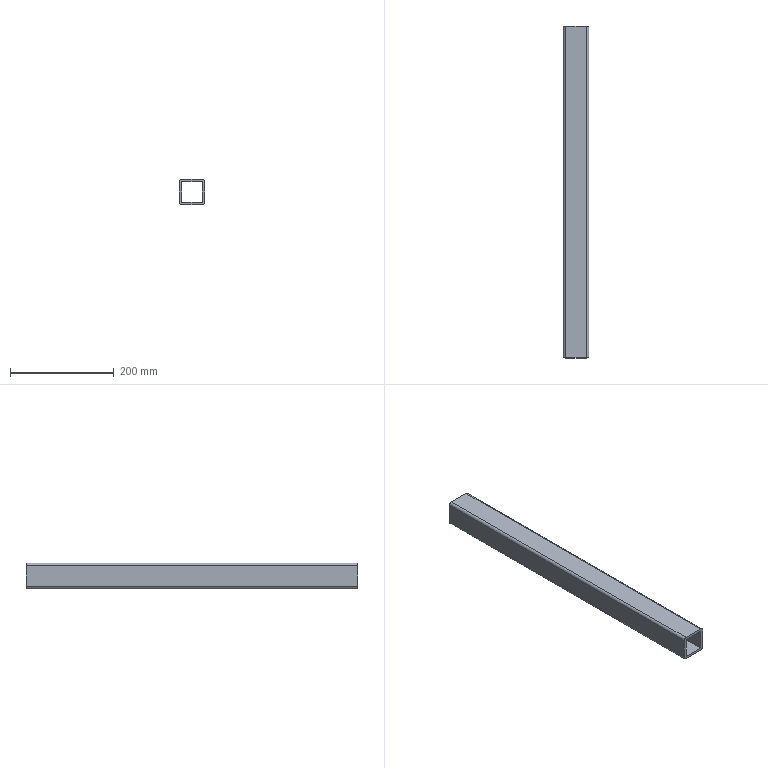Part | STEP file | 50x50x640 | 1 solid | 14 faces | box 50 x 640 x 50 mm | volume 562265 mm3 | plane 10 | cylinder 4 | commonest cylinder face diameters 10 x4
STEP:
#1=CARTESIAN_POINT('',(0.,0.,0.));
#2=DIRECTION('',(0.,0.,1.));
#3=DIRECTION('',(1.,0.,0.));
#4=AXIS2_PLACEMENT_3D('',#1,#2,#3);
#5=CARTESIAN_POINT('',(-758.5,-265.,-25.));
#6=VERTEX_POINT('',#5);
#7=CARTESIAN_POINT('',(-758.5,-265.,-65.));
#8=VERTEX_POINT('',#7);
#9=CARTESIAN_POINT('',(-758.5,-265.,-65.));
#10=DIRECTION('',(0.,0.,-1.));
#11=VECTOR('',#10,1.);
#12=LINE('',#9,#11);
#13=CARTESIAN_POINT('',(-758.5,845.,-65.));
#14=DIRECTION('',(-1.,0.,0.));
#15=DIRECTION('',(0.,0.,-1.));
#16=AXIS2_PLACEMENT_3D('',#13,#14,#15);
#17=PLANE('',#16);
#18=CARTESIAN_POINT('',(0.,1110.));
#19=DIRECTION('',(1.,0.));
#20=VECTOR('',#19,1.);
#21=LINE('',#18,#20);
#22=(GEOMETRIC_REPRESENTATION_CONTEXT(2)PARAMETRIC_REPRESENTATION_CONTEXT()REPRESENTATION_CONTEXT('',''));
#23=DEFINITIONAL_REPRESENTATION('',(#21),#22);
#24=PCURVE('',#17,#23);
#25=CARTESIAN_POINT('',(666.5,-265.,-65.));
#26=DIRECTION('',(0.,-1.,0.));
#27=DIRECTION('',(0.,0.,-1.));
#28=AXIS2_PLACEMENT_3D('',#25,#26,#27);
#29=PLANE('',#28);
#30=CARTESIAN_POINT('',(0.,-1425.));
#31=DIRECTION('',(1.,0.));
#32=VECTOR('',#31,1.);
#33=LINE('',#30,#32);
#34=(GEOMETRIC_REPRESENTATION_CONTEXT(2)PARAMETRIC_REPRESENTATION_CONTEXT()REPRESENTATION_CONTEXT('',''));
#35=DEFINITIONAL_REPRESENTATION('',(#33),#34);
#36=PCURVE('',#29,#35);
#37=SURFACE_CURVE('',#12,(#24,#36),.PCURVE_S1.);
#38=EDGE_CURVE('',#6,#8,#37,.T.);
#39=ORIENTED_EDGE('',*,*,#38,.F.);
#40=CARTESIAN_POINT('',(-758.5,375.,-25.));
#41=VERTEX_POINT('',#40);
#42=CARTESIAN_POINT('',(-758.5,845.,-25.));
#43=DIRECTION('',(0.,1.,0.));
#44=VECTOR('',#43,1.);
#45=LINE('',#42,#44);
#46=CARTESIAN_POINT('',(-40.,0.));
#47=DIRECTION('',(0.,-1.));
#48=VECTOR('',#47,1.);
#49=LINE('',#46,#48);
#50=(GEOMETRIC_REPRESENTATION_CONTEXT(2)PARAMETRIC_REPRESENTATION_CONTEXT()REPRESENTATION_CONTEXT('',''));
#51=DEFINITIONAL_REPRESENTATION('',(#49),#50);
#52=PCURVE('',#17,#51);
#53=CARTESIAN_POINT('',(-758.5,845.,-25.));
#54=DIRECTION('',(0.,0.,-1.));
#55=DIRECTION('',(1.,0.,0.));
#56=AXIS2_PLACEMENT_3D('',#53,#54,#55);
#57=PLANE('',#56);
#58=CARTESIAN_POINT('',(0.,0.));
#59=DIRECTION('',(0.,-1.));
#60=VECTOR('',#59,1.);
#61=LINE('',#58,#60);
#62=(GEOMETRIC_REPRESENTATION_CONTEXT(2)PARAMETRIC_REPRESENTATION_CONTEXT()REPRESENTATION_CONTEXT('',''));
#63=DEFINITIONAL_REPRESENTATION('',(#61),#62);
#64=PCURVE('',#57,#63);
#65=SURFACE_CURVE('',#45,(#52,#64),.PCURVE_S1.);
#66=EDGE_CURVE('',#6,#41,#65,.T.);
#67=ORIENTED_EDGE('',*,*,#66,.T.);
#68=CARTESIAN_POINT('',(-758.5,375.,-65.));
#69=VERTEX_POINT('',#68);
#70=CARTESIAN_POINT('',(-758.5,375.,-65.));
#71=DIRECTION('',(0.,0.,-1.));
#72=VECTOR('',#71,1.);
#73=LINE('',#70,#72);
#74=CARTESIAN_POINT('',(0.,470.));
#75=DIRECTION('',(1.,0.));
#76=VECTOR('',#75,1.);
#77=LINE('',#74,#76);
#78=(GEOMETRIC_REPRESENTATION_CONTEXT(2)PARAMETRIC_REPRESENTATION_CONTEXT()REPRESENTATION_CONTEXT('',''));
#79=DEFINITIONAL_REPRESENTATION('',(#77),#78);
#80=PCURVE('',#17,#79);
#81=CARTESIAN_POINT('',(-1003.5,375.,-65.));
#82=DIRECTION('',(0.,1.,0.));
#83=DIRECTION('',(0.,0.,-1.));
#84=AXIS2_PLACEMENT_3D('',#81,#82,#83);
#85=PLANE('',#84);
#86=CARTESIAN_POINT('',(0.,-245.));
#87=DIRECTION('',(1.,0.));
#88=VECTOR('',#87,1.);
#89=LINE('',#86,#88);
#90=(GEOMETRIC_REPRESENTATION_CONTEXT(2)PARAMETRIC_REPRESENTATION_CONTEXT()REPRESENTATION_CONTEXT('',''));
#91=DEFINITIONAL_REPRESENTATION('',(#89),#90);
#92=PCURVE('',#85,#91);
#93=SURFACE_CURVE('',#73,(#80,#92),.PCURVE_S1.);
#94=EDGE_CURVE('',#41,#69,#93,.T.);
#95=ORIENTED_EDGE('',*,*,#94,.T.);
#96=CARTESIAN_POINT('',(-758.5,845.,-65.));
#97=DIRECTION('',(0.,1.,0.));
#98=VECTOR('',#97,1.);
#99=LINE('',#96,#98);
#100=CARTESIAN_POINT('',(0.,0.));
#101=DIRECTION('',(0.,-1.));
#102=VECTOR('',#101,1.);
#103=LINE('',#100,#102);
#104=(GEOMETRIC_REPRESENTATION_CONTEXT(2)PARAMETRIC_REPRESENTATION_CONTEXT()REPRESENTATION_CONTEXT('',''));
#105=DEFINITIONAL_REPRESENTATION('',(#103),#104);
#106=PCURVE('',#17,#105);
#107=CARTESIAN_POINT('',(-798.5,845.,-65.));
#108=DIRECTION('',(0.,0.,1.));
#109=DIRECTION('',(-1.,0.,0.));
#110=AXIS2_PLACEMENT_3D('',#107,#108,#109);
#111=PLANE('',#110);
#112=CARTESIAN_POINT('',(-40.,0.));
#113=DIRECTION('',(0.,-1.));
#114=VECTOR('',#113,1.);
#115=LINE('',#112,#114);
#116=(GEOMETRIC_REPRESENTATION_CONTEXT(2)PARAMETRIC_REPRESENTATION_CONTEXT()REPRESENTATION_CONTEXT('',''));
#117=DEFINITIONAL_REPRESENTATION('',(#115),#116);
#118=PCURVE('',#111,#117);
#119=SURFACE_CURVE('',#99,(#106,#118),.PCURVE_S1.);
#120=EDGE_CURVE('',#8,#69,#119,.T.);
#121=ORIENTED_EDGE('',*,*,#120,.F.);
#122=EDGE_LOOP('',(#39,#67,#95,#121));
#123=FACE_BOUND('',#122,.T.);
#124=ADVANCED_FACE('',(#123),#17,.T.);
#125=CARTESIAN_POINT('',(-798.5,-265.,-25.));
#126=VERTEX_POINT('',#125);
#127=CARTESIAN_POINT('',(666.5,-265.,-25.));
#128=DIRECTION('',(1.,0.,0.));
#129=VECTOR('',#128,1.);
#130=LINE('',#127,#129);
#131=CARTESIAN_POINT('',(1425.,1110.));
#132=DIRECTION('',(1.,0.));
#133=VECTOR('',#132,1.);
#134=LINE('',#131,#133);
#135=(GEOMETRIC_REPRESENTATION_CONTEXT(2)PARAMETRIC_REPRESENTATION_CONTEXT()REPRESENTATION_CONTEXT('',''));
#136=DEFINITIONAL_REPRESENTATION('',(#134),#135);
#137=PCURVE('',#57,#136);
#138=CARTESIAN_POINT('',(-40.,0.));
#139=DIRECTION('',(0.,1.));
#140=VECTOR('',#139,1.);
#141=LINE('',#138,#140);
#142=(GEOMETRIC_REPRESENTATION_CONTEXT(2)PARAMETRIC_REPRESENTATION_CONTEXT()REPRESENTATION_CONTEXT('',''));
#143=DEFINITIONAL_REPRESENTATION('',(#141),#142);
#144=PCURVE('',#29,#143);
#145=SURFACE_CURVE('',#130,(#137,#144),.PCURVE_S1.);
#146=EDGE_CURVE('',#126,#6,#145,.T.);
#147=ORIENTED_EDGE('',*,*,#146,.F.);
#148=CARTESIAN_POINT('',(-798.5,375.,-25.));
#149=VERTEX_POINT('',#148);
#150=CARTESIAN_POINT('',(-798.5,845.,-25.));
#151=DIRECTION('',(0.,1.,0.));
#152=VECTOR('',#151,1.);
#153=LINE('',#150,#152);
#154=CARTESIAN_POINT('',(-40.,0.));
#155=DIRECTION('',(0.,-1.));
#156=VECTOR('',#155,1.);
#157=LINE('',#154,#156);
#158=(GEOMETRIC_REPRESENTATION_CONTEXT(2)PARAMETRIC_REPRESENTATION_CONTEXT()REPRESENTATION_CONTEXT('',''));
#159=DEFINITIONAL_REPRESENTATION('',(#157),#158);
#160=PCURVE('',#57,#159);
#161=CARTESIAN_POINT('',(-798.5,845.,-25.));
#162=DIRECTION('',(1.,0.,0.));
#163=DIRECTION('',(0.,0.,1.));
#164=AXIS2_PLACEMENT_3D('',#161,#162,#163);
#165=PLANE('',#164);
#166=CARTESIAN_POINT('',(0.,0.));
#167=DIRECTION('',(0.,-1.));
#168=VECTOR('',#167,1.);
#169=LINE('',#166,#168);
#170=(GEOMETRIC_REPRESENTATION_CONTEXT(2)PARAMETRIC_REPRESENTATION_CONTEXT()REPRESENTATION_CONTEXT('',''));
#171=DEFINITIONAL_REPRESENTATION('',(#169),#170);
#172=PCURVE('',#165,#171);
#173=SURFACE_CURVE('',#153,(#160,#172),.PCURVE_S1.);
#174=EDGE_CURVE('',#126,#149,#173,.T.);
#175=ORIENTED_EDGE('',*,*,#174,.T.);
#176=CARTESIAN_POINT('',(-1003.5,375.,-25.));
#177=DIRECTION('',(1.,0.,0.));
#178=VECTOR('',#177,1.);
#179=LINE('',#176,#178);
#180=CARTESIAN_POINT('',(-245.,470.));
#181=DIRECTION('',(1.,0.));
#182=VECTOR('',#181,1.);
#183=LINE('',#180,#182);
#184=(GEOMETRIC_REPRESENTATION_CONTEXT(2)PARAMETRIC_REPRESENTATION_CONTEXT()REPRESENTATION_CONTEXT('',''));
#185=DEFINITIONAL_REPRESENTATION('',(#183),#184);
#186=PCURVE('',#57,#185);
#187=CARTESIAN_POINT('',(-40.,0.));
#188=DIRECTION('',(0.,-1.));
#189=VECTOR('',#188,1.);
#190=LINE('',#187,#189);
#191=(GEOMETRIC_REPRESENTATION_CONTEXT(2)PARAMETRIC_REPRESENTATION_CONTEXT()REPRESENTATION_CONTEXT('',''));
#192=DEFINITIONAL_REPRESENTATION('',(#190),#191);
#193=PCURVE('',#85,#192);
#194=SURFACE_CURVE('',#179,(#186,#193),.PCURVE_S1.);
#195=EDGE_CURVE('',#149,#41,#194,.T.);
#196=ORIENTED_EDGE('',*,*,#195,.T.);
#197=ORIENTED_EDGE('',*,*,#66,.F.);
#198=EDGE_LOOP('',(#147,#175,#196,#197));
#199=FACE_BOUND('',#198,.T.);
#200=ADVANCED_FACE('',(#199),#57,.T.);
#201=CARTESIAN_POINT('',(-798.5,-265.,-65.));
#202=VERTEX_POINT('',#201);
#203=CARTESIAN_POINT('',(-798.5,-265.,-65.));
#204=DIRECTION('',(0.,0.,1.));
#205=VECTOR('',#204,1.);
#206=LINE('',#203,#205);
#207=CARTESIAN_POINT('',(-40.,1110.));
#208=DIRECTION('',(1.,0.));
#209=VECTOR('',#208,1.);
#210=LINE('',#207,#209);
#211=(GEOMETRIC_REPRESENTATION_CONTEXT(2)PARAMETRIC_REPRESENTATION_CONTEXT()REPRESENTATION_CONTEXT('',''));
#212=DEFINITIONAL_REPRESENTATION('',(#210),#211);
#213=PCURVE('',#165,#212);
#214=CARTESIAN_POINT('',(0.,-1465.));
#215=DIRECTION('',(-1.,0.));
#216=VECTOR('',#215,1.);
#217=LINE('',#214,#216);
#218=(GEOMETRIC_REPRESENTATION_CONTEXT(2)PARAMETRIC_REPRESENTATION_CONTEXT()REPRESENTATION_CONTEXT('',''));
#219=DEFINITIONAL_REPRESENTATION('',(#217),#218);
#220=PCURVE('',#29,#219);
#221=SURFACE_CURVE('',#206,(#213,#220),.PCURVE_S1.);
#222=EDGE_CURVE('',#202,#126,#221,.T.);
#223=ORIENTED_EDGE('',*,*,#222,.F.);
#224=CARTESIAN_POINT('',(-798.5,375.,-65.));
#225=VERTEX_POINT('',#224);
#226=CARTESIAN_POINT('',(-798.5,845.,-65.));
#227=DIRECTION('',(0.,1.,0.));
#228=VECTOR('',#227,1.);
#229=LINE('',#226,#228);
#230=CARTESIAN_POINT('',(-40.,0.));
#231=DIRECTION('',(0.,-1.));
#232=VECTOR('',#231,1.);
#233=LINE('',#230,#232);
#234=(GEOMETRIC_REPRESENTATION_CONTEXT(2)PARAMETRIC_REPRESENTATION_CONTEXT()REPRESENTATION_CONTEXT('',''));
#235=DEFINITIONAL_REPRESENTATION('',(#233),#234);
#236=PCURVE('',#165,#235);
#237=CARTESIAN_POINT('',(0.,0.));
#238=DIRECTION('',(0.,-1.));
#239=VECTOR('',#238,1.);
#240=LINE('',#237,#239);
#241=(GEOMETRIC_REPRESENTATION_CONTEXT(2)PARAMETRIC_REPRESENTATION_CONTEXT()REPRESENTATION_CONTEXT('',''));
#242=DEFINITIONAL_REPRESENTATION('',(#240),#241);
#243=PCURVE('',#111,#242);
#244=SURFACE_CURVE('',#229,(#236,#243),.PCURVE_S1.);
#245=EDGE_CURVE('',#202,#225,#244,.T.);
#246=ORIENTED_EDGE('',*,*,#245,.T.);
#247=CARTESIAN_POINT('',(-798.5,375.,-65.));
#248=DIRECTION('',(0.,0.,1.));
#249=VECTOR('',#248,1.);
#250=LINE('',#247,#249);
#251=CARTESIAN_POINT('',(-40.,470.));
#252=DIRECTION('',(1.,0.));
#253=VECTOR('',#252,1.);
#254=LINE('',#251,#253);
#255=(GEOMETRIC_REPRESENTATION_CONTEXT(2)PARAMETRIC_REPRESENTATION_CONTEXT()REPRESENTATION_CONTEXT('',''));
#256=DEFINITIONAL_REPRESENTATION('',(#254),#255);
#257=PCURVE('',#165,#256);
#258=CARTESIAN_POINT('',(0.,-205.));
#259=DIRECTION('',(-1.,0.));
#260=VECTOR('',#259,1.);
#261=LINE('',#258,#260);
#262=(GEOMETRIC_REPRESENTATION_CONTEXT(2)PARAMETRIC_REPRESENTATION_CONTEXT()REPRESENTATION_CONTEXT('',''));
#263=DEFINITIONAL_REPRESENTATION('',(#261),#262);
#264=PCURVE('',#85,#263);
#265=SURFACE_CURVE('',#250,(#257,#264),.PCURVE_S1.);
#266=EDGE_CURVE('',#225,#149,#265,.T.);
#267=ORIENTED_EDGE('',*,*,#266,.T.);
#268=ORIENTED_EDGE('',*,*,#174,.F.);
#269=EDGE_LOOP('',(#223,#246,#267,#268));
#270=FACE_BOUND('',#269,.T.);
#271=ADVANCED_FACE('',(#270),#165,.T.);
#272=CARTESIAN_POINT('',(-753.5,-265.,-65.));
#273=VERTEX_POINT('',#272);
#274=CARTESIAN_POINT('',(-753.5,-265.,-25.));
#275=VERTEX_POINT('',#274);
#276=CARTESIAN_POINT('',(-753.5,-265.,-65.));
#277=DIRECTION('',(0.,0.,1.));
#278=VECTOR('',#277,1.);
#279=LINE('',#276,#278);
#280=CARTESIAN_POINT('',(-753.5,845.,-25.));
#281=DIRECTION('',(1.,0.,0.));
#282=DIRECTION('',(0.,0.,1.));
#283=AXIS2_PLACEMENT_3D('',#280,#281,#282);
#284=PLANE('',#283);
#285=CARTESIAN_POINT('',(-40.,1110.));
#286=DIRECTION('',(1.,0.));
#287=VECTOR('',#286,1.);
#288=LINE('',#285,#287);
#289=(GEOMETRIC_REPRESENTATION_CONTEXT(2)PARAMETRIC_REPRESENTATION_CONTEXT()REPRESENTATION_CONTEXT('',''));
#290=DEFINITIONAL_REPRESENTATION('',(#288),#289);
#291=PCURVE('',#284,#290);
#292=CARTESIAN_POINT('',(0.,-1420.));
#293=DIRECTION('',(-1.,0.));
#294=VECTOR('',#293,1.);
#295=LINE('',#292,#294);
#296=(GEOMETRIC_REPRESENTATION_CONTEXT(2)PARAMETRIC_REPRESENTATION_CONTEXT()REPRESENTATION_CONTEXT('',''));
#297=DEFINITIONAL_REPRESENTATION('',(#295),#296);
#298=PCURVE('',#29,#297);
#299=SURFACE_CURVE('',#279,(#291,#298),.PCURVE_S1.);
#300=EDGE_CURVE('',#273,#275,#299,.T.);
#301=ORIENTED_EDGE('',*,*,#300,.F.);
#302=CARTESIAN_POINT('',(-753.5,375.,-65.));
#303=VERTEX_POINT('',#302);
#304=CARTESIAN_POINT('',(-753.5,845.,-65.));
#305=DIRECTION('',(0.,1.,0.));
#306=VECTOR('',#305,1.);
#307=LINE('',#304,#306);
#308=CARTESIAN_POINT('',(-40.,0.));
#309=DIRECTION('',(0.,-1.));
#310=VECTOR('',#309,1.);
#311=LINE('',#308,#310);
#312=(GEOMETRIC_REPRESENTATION_CONTEXT(2)PARAMETRIC_REPRESENTATION_CONTEXT()REPRESENTATION_CONTEXT('',''));
#313=DEFINITIONAL_REPRESENTATION('',(#311),#312);
#314=PCURVE('',#284,#313);
#315=CARTESIAN_POINT('',(-758.5,845.,-65.));
#316=DIRECTION('',(0.,-1.,0.));
#317=DIRECTION('',(0.,0.,-1.));
#318=AXIS2_PLACEMENT_3D('',#315,#316,#317);
#319=CYLINDRICAL_SURFACE('',#318,5.);
#320=CARTESIAN_POINT('',(1.571,0.));
#321=DIRECTION('',(0.,-1.));
#322=VECTOR('',#321,1.);
#323=LINE('',#320,#322);
#324=(GEOMETRIC_REPRESENTATION_CONTEXT(2)PARAMETRIC_REPRESENTATION_CONTEXT()REPRESENTATION_CONTEXT('',''));
#325=DEFINITIONAL_REPRESENTATION('',(#323),#324);
#326=PCURVE('',#319,#325);
#327=SURFACE_CURVE('',#307,(#314,#326),.PCURVE_S1.);
#328=EDGE_CURVE('',#273,#303,#327,.T.);
#329=ORIENTED_EDGE('',*,*,#328,.T.);
#330=CARTESIAN_POINT('',(-753.5,375.,-25.));
#331=VERTEX_POINT('',#330);
#332=CARTESIAN_POINT('',(-753.5,375.,-65.));
#333=DIRECTION('',(0.,0.,1.));
#334=VECTOR('',#333,1.);
#335=LINE('',#332,#334);
#336=CARTESIAN_POINT('',(-40.,470.));
#337=DIRECTION('',(1.,0.));
#338=VECTOR('',#337,1.);
#339=LINE('',#336,#338);
#340=(GEOMETRIC_REPRESENTATION_CONTEXT(2)PARAMETRIC_REPRESENTATION_CONTEXT()REPRESENTATION_CONTEXT('',''));
#341=DEFINITIONAL_REPRESENTATION('',(#339),#340);
#342=PCURVE('',#284,#341);
#343=CARTESIAN_POINT('',(0.,-250.));
#344=DIRECTION('',(-1.,0.));
#345=VECTOR('',#344,1.);
#346=LINE('',#343,#345);
#347=(GEOMETRIC_REPRESENTATION_CONTEXT(2)PARAMETRIC_REPRESENTATION_CONTEXT()REPRESENTATION_CONTEXT('',''));
#348=DEFINITIONAL_REPRESENTATION('',(#346),#347);
#349=PCURVE('',#85,#348);
#350=SURFACE_CURVE('',#335,(#342,#349),.PCURVE_S1.);
#351=EDGE_CURVE('',#303,#331,#350,.T.);
#352=ORIENTED_EDGE('',*,*,#351,.T.);
#353=CARTESIAN_POINT('',(-753.5,845.,-25.));
#354=DIRECTION('',(0.,1.,0.));
#355=VECTOR('',#354,1.);
#356=LINE('',#353,#355);
#357=CARTESIAN_POINT('',(0.,0.));
#358=DIRECTION('',(0.,-1.));
#359=VECTOR('',#358,1.);
#360=LINE('',#357,#359);
#361=(GEOMETRIC_REPRESENTATION_CONTEXT(2)PARAMETRIC_REPRESENTATION_CONTEXT()REPRESENTATION_CONTEXT('',''));
#362=DEFINITIONAL_REPRESENTATION('',(#360),#361);
#363=PCURVE('',#284,#362);
#364=CARTESIAN_POINT('',(-758.5,845.,-25.));
#365=DIRECTION('',(0.,-1.,0.));
#366=DIRECTION('',(0.,0.,-1.));
#367=AXIS2_PLACEMENT_3D('',#364,#365,#366);
#368=CYLINDRICAL_SURFACE('',#367,5.);
#369=CARTESIAN_POINT('',(1.571,0.));
#370=DIRECTION('',(0.,-1.));
#371=VECTOR('',#370,1.);
#372=LINE('',#369,#371);
#373=(GEOMETRIC_REPRESENTATION_CONTEXT(2)PARAMETRIC_REPRESENTATION_CONTEXT()REPRESENTATION_CONTEXT('',''));
#374=DEFINITIONAL_REPRESENTATION('',(#372),#373);
#375=PCURVE('',#368,#374);
#376=SURFACE_CURVE('',#356,(#363,#375),.PCURVE_S1.);
#377=EDGE_CURVE('',#275,#331,#376,.T.);
#378=ORIENTED_EDGE('',*,*,#377,.F.);
#379=EDGE_LOOP('',(#301,#329,#352,#378));
#380=FACE_BOUND('',#379,.T.);
#381=ADVANCED_FACE('',(#380),#284,.T.);
#382=CARTESIAN_POINT('',(-758.5,-265.,-70.));
#383=VERTEX_POINT('',#382);
#384=CARTESIAN_POINT('',(-758.5,-265.,-65.));
#385=DIRECTION('',(0.,-1.,0.));
#386=DIRECTION('',(0.,0.,-1.));
#387=AXIS2_PLACEMENT_3D('',#384,#385,#386);
#388=CIRCLE('',#387,5.);
#389=CARTESIAN_POINT('',(0.,1110.));
#390=DIRECTION('',(1.,0.));
#391=VECTOR('',#390,1.);
#392=LINE('',#389,#391);
#393=(GEOMETRIC_REPRESENTATION_CONTEXT(2)PARAMETRIC_REPRESENTATION_CONTEXT()REPRESENTATION_CONTEXT('',''));
#394=DEFINITIONAL_REPRESENTATION('',(#392),#393);
#395=PCURVE('',#319,#394);
#396=CARTESIAN_POINT('',(0.,-1425.));
#397=DIRECTION('',(1.,0.));
#398=AXIS2_PLACEMENT_2D('',#396,#397);
#399=CIRCLE('',#398,5.);
#400=(GEOMETRIC_REPRESENTATION_CONTEXT(2)PARAMETRIC_REPRESENTATION_CONTEXT()REPRESENTATION_CONTEXT('',''));
#401=DEFINITIONAL_REPRESENTATION('',(#399),#400);
#402=PCURVE('',#29,#401);
#403=SURFACE_CURVE('',#388,(#395,#402),.PCURVE_S1.);
#404=EDGE_CURVE('',#383,#273,#403,.T.);
#405=ORIENTED_EDGE('',*,*,#404,.F.);
#406=CARTESIAN_POINT('',(-758.5,375.,-70.));
#407=VERTEX_POINT('',#406);
#408=CARTESIAN_POINT('',(-758.5,845.,-70.));
#409=DIRECTION('',(0.,1.,0.));
#410=VECTOR('',#409,1.);
#411=LINE('',#408,#410);
#412=CARTESIAN_POINT('',(0.,0.));
#413=DIRECTION('',(0.,-1.));
#414=VECTOR('',#413,1.);
#415=LINE('',#412,#414);
#416=(GEOMETRIC_REPRESENTATION_CONTEXT(2)PARAMETRIC_REPRESENTATION_CONTEXT()REPRESENTATION_CONTEXT('',''));
#417=DEFINITIONAL_REPRESENTATION('',(#415),#416);
#418=PCURVE('',#319,#417);
#419=CARTESIAN_POINT('',(-758.5,845.,-70.));
#420=DIRECTION('',(0.,0.,-1.));
#421=DIRECTION('',(1.,0.,0.));
#422=AXIS2_PLACEMENT_3D('',#419,#420,#421);
#423=PLANE('',#422);
#424=CARTESIAN_POINT('',(0.,0.));
#425=DIRECTION('',(0.,-1.));
#426=VECTOR('',#425,1.);
#427=LINE('',#424,#426);
#428=(GEOMETRIC_REPRESENTATION_CONTEXT(2)PARAMETRIC_REPRESENTATION_CONTEXT()REPRESENTATION_CONTEXT('',''));
#429=DEFINITIONAL_REPRESENTATION('',(#427),#428);
#430=PCURVE('',#423,#429);
#431=SURFACE_CURVE('',#411,(#418,#430),.PCURVE_S1.);
#432=EDGE_CURVE('',#383,#407,#431,.T.);
#433=ORIENTED_EDGE('',*,*,#432,.T.);
#434=CARTESIAN_POINT('',(-758.5,375.,-65.));
#435=DIRECTION('',(0.,-1.,0.));
#436=DIRECTION('',(0.,0.,1.));
#437=AXIS2_PLACEMENT_3D('',#434,#435,#436);
#438=CIRCLE('',#437,5.);
#439=CARTESIAN_POINT('',(-3.142,470.));
#440=DIRECTION('',(1.,0.));
#441=VECTOR('',#440,1.);
#442=LINE('',#439,#441);
#443=(GEOMETRIC_REPRESENTATION_CONTEXT(2)PARAMETRIC_REPRESENTATION_CONTEXT()REPRESENTATION_CONTEXT('',''));
#444=DEFINITIONAL_REPRESENTATION('',(#442),#443);
#445=PCURVE('',#319,#444);
#446=CARTESIAN_POINT('',(-5.,-245.));
#447=CARTESIAN_POINT('',(-5.,-236.34));
#448=CARTESIAN_POINT('',(2.5,-240.67));
#449=CARTESIAN_POINT('',(10.,-245.));
#450=CARTESIAN_POINT('',(2.5,-249.33));
#451=CARTESIAN_POINT('',(-5.,-253.66));
#452=CARTESIAN_POINT('',(-5.,-245.));
#453=(BOUNDED_CURVE()B_SPLINE_CURVE(2,(#446,#447,#448,#449,#450,#451,#452),.UNSPECIFIED.,.T.,.F.)B_SPLINE_CURVE_WITH_KNOTS((1,2,2,2,2,1),(-2.094,0.,2.094,4.189,6.283,8.378),.UNSPECIFIED.)CURVE()GEOMETRIC_REPRESENTATION_ITEM()RATIONAL_B_SPLINE_CURVE((1.,0.5,1.,0.5,1.,0.5,1.))REPRESENTATION_ITEM(''));
#454=(GEOMETRIC_REPRESENTATION_CONTEXT(2)PARAMETRIC_REPRESENTATION_CONTEXT()REPRESENTATION_CONTEXT('',''));
#455=DEFINITIONAL_REPRESENTATION('',(#453),#454);
#456=PCURVE('',#85,#455);
#457=SURFACE_CURVE('',#438,(#445,#456),.PCURVE_S1.);
#458=EDGE_CURVE('',#407,#303,#457,.T.);
#459=ORIENTED_EDGE('',*,*,#458,.T.);
#460=ORIENTED_EDGE('',*,*,#328,.F.);
#461=EDGE_LOOP('',(#405,#433,#459,#460));
#462=FACE_BOUND('',#461,.T.);
#463=ADVANCED_FACE('',(#462),#319,.T.);
#464=CARTESIAN_POINT('',(-798.5,-265.,-70.));
#465=VERTEX_POINT('',#464);
#466=CARTESIAN_POINT('',(666.5,-265.,-70.));
#467=DIRECTION('',(1.,0.,0.));
#468=VECTOR('',#467,1.);
#469=LINE('',#466,#468);
#470=CARTESIAN_POINT('',(1425.,1110.));
#471=DIRECTION('',(1.,0.));
#472=VECTOR('',#471,1.);
#473=LINE('',#470,#472);
#474=(GEOMETRIC_REPRESENTATION_CONTEXT(2)PARAMETRIC_REPRESENTATION_CONTEXT()REPRESENTATION_CONTEXT('',''));
#475=DEFINITIONAL_REPRESENTATION('',(#473),#474);
#476=PCURVE('',#423,#475);
#477=CARTESIAN_POINT('',(5.,0.));
#478=DIRECTION('',(0.,1.));
#479=VECTOR('',#478,1.);
#480=LINE('',#477,#479);
#481=(GEOMETRIC_REPRESENTATION_CONTEXT(2)PARAMETRIC_REPRESENTATION_CONTEXT()REPRESENTATION_CONTEXT('',''));
#482=DEFINITIONAL_REPRESENTATION('',(#480),#481);
#483=PCURVE('',#29,#482);
#484=SURFACE_CURVE('',#469,(#476,#483),.PCURVE_S1.);
#485=EDGE_CURVE('',#465,#383,#484,.T.);
#486=ORIENTED_EDGE('',*,*,#485,.F.);
#487=CARTESIAN_POINT('',(-798.5,375.,-70.));
#488=VERTEX_POINT('',#487);
#489=CARTESIAN_POINT('',(-798.5,845.,-70.));
#490=DIRECTION('',(0.,1.,0.));
#491=VECTOR('',#490,1.);
#492=LINE('',#489,#491);
#493=CARTESIAN_POINT('',(-40.,0.));
#494=DIRECTION('',(0.,-1.));
#495=VECTOR('',#494,1.);
#496=LINE('',#493,#495);
#497=(GEOMETRIC_REPRESENTATION_CONTEXT(2)PARAMETRIC_REPRESENTATION_CONTEXT()REPRESENTATION_CONTEXT('',''));
#498=DEFINITIONAL_REPRESENTATION('',(#496),#497);
#499=PCURVE('',#423,#498);
#500=CARTESIAN_POINT('',(-798.5,845.,-65.));
#501=DIRECTION('',(0.,-1.,0.));
#502=DIRECTION('',(0.,0.,-1.));
#503=AXIS2_PLACEMENT_3D('',#500,#501,#502);
#504=CYLINDRICAL_SURFACE('',#503,5.);
#505=CARTESIAN_POINT('',(6.283,0.));
#506=DIRECTION('',(0.,-1.));
#507=VECTOR('',#506,1.);
#508=LINE('',#505,#507);
#509=(GEOMETRIC_REPRESENTATION_CONTEXT(2)PARAMETRIC_REPRESENTATION_CONTEXT()REPRESENTATION_CONTEXT('',''));
#510=DEFINITIONAL_REPRESENTATION('',(#508),#509);
#511=PCURVE('',#504,#510);
#512=SURFACE_CURVE('',#492,(#499,#511),.PCURVE_S1.);
#513=EDGE_CURVE('',#465,#488,#512,.T.);
#514=ORIENTED_EDGE('',*,*,#513,.T.);
#515=CARTESIAN_POINT('',(-1003.5,375.,-70.));
#516=DIRECTION('',(1.,0.,0.));
#517=VECTOR('',#516,1.);
#518=LINE('',#515,#517);
#519=CARTESIAN_POINT('',(-245.,470.));
#520=DIRECTION('',(1.,0.));
#521=VECTOR('',#520,1.);
#522=LINE('',#519,#521);
#523=(GEOMETRIC_REPRESENTATION_CONTEXT(2)PARAMETRIC_REPRESENTATION_CONTEXT()REPRESENTATION_CONTEXT('',''));
#524=DEFINITIONAL_REPRESENTATION('',(#522),#523);
#525=PCURVE('',#423,#524);
#526=CARTESIAN_POINT('',(5.,0.));
#527=DIRECTION('',(0.,-1.));
#528=VECTOR('',#527,1.);
#529=LINE('',#526,#528);
#530=(GEOMETRIC_REPRESENTATION_CONTEXT(2)PARAMETRIC_REPRESENTATION_CONTEXT()REPRESENTATION_CONTEXT('',''));
#531=DEFINITIONAL_REPRESENTATION('',(#529),#530);
#532=PCURVE('',#85,#531);
#533=SURFACE_CURVE('',#518,(#525,#532),.PCURVE_S1.);
#534=EDGE_CURVE('',#488,#407,#533,.T.);
#535=ORIENTED_EDGE('',*,*,#534,.T.);
#536=ORIENTED_EDGE('',*,*,#432,.F.);
#537=EDGE_LOOP('',(#486,#514,#535,#536));
#538=FACE_BOUND('',#537,.T.);
#539=ADVANCED_FACE('',(#538),#423,.T.);
#540=CARTESIAN_POINT('',(-803.5,-265.,-65.));
#541=VERTEX_POINT('',#540);
#542=CARTESIAN_POINT('',(-798.5,-265.,-65.));
#543=DIRECTION('',(0.,-1.,0.));
#544=DIRECTION('',(0.,0.,-1.));
#545=AXIS2_PLACEMENT_3D('',#542,#543,#544);
#546=CIRCLE('',#545,5.);
#547=CARTESIAN_POINT('',(0.,1110.));
#548=DIRECTION('',(1.,0.));
#549=VECTOR('',#548,1.);
#550=LINE('',#547,#549);
#551=(GEOMETRIC_REPRESENTATION_CONTEXT(2)PARAMETRIC_REPRESENTATION_CONTEXT()REPRESENTATION_CONTEXT('',''));
#552=DEFINITIONAL_REPRESENTATION('',(#550),#551);
#553=PCURVE('',#504,#552);
#554=CARTESIAN_POINT('',(0.,-1465.));
#555=DIRECTION('',(1.,0.));
#556=AXIS2_PLACEMENT_2D('',#554,#555);
#557=CIRCLE('',#556,5.);
#558=(GEOMETRIC_REPRESENTATION_CONTEXT(2)PARAMETRIC_REPRESENTATION_CONTEXT()REPRESENTATION_CONTEXT('',''));
#559=DEFINITIONAL_REPRESENTATION('',(#557),#558);
#560=PCURVE('',#29,#559);
#561=SURFACE_CURVE('',#546,(#553,#560),.PCURVE_S1.);
#562=EDGE_CURVE('',#541,#465,#561,.T.);
#563=ORIENTED_EDGE('',*,*,#562,.F.);
#564=CARTESIAN_POINT('',(-803.5,375.,-65.));
#565=VERTEX_POINT('',#564);
#566=CARTESIAN_POINT('',(-803.5,845.,-65.));
#567=DIRECTION('',(0.,1.,0.));
#568=VECTOR('',#567,1.);
#569=LINE('',#566,#568);
#570=CARTESIAN_POINT('',(4.712,0.));
#571=DIRECTION('',(0.,-1.));
#572=VECTOR('',#571,1.);
#573=LINE('',#570,#572);
#574=(GEOMETRIC_REPRESENTATION_CONTEXT(2)PARAMETRIC_REPRESENTATION_CONTEXT()REPRESENTATION_CONTEXT('',''));
#575=DEFINITIONAL_REPRESENTATION('',(#573),#574);
#576=PCURVE('',#504,#575);
#577=CARTESIAN_POINT('',(-803.5,845.,-65.));
#578=DIRECTION('',(-1.,0.,0.));
#579=DIRECTION('',(0.,0.,-1.));
#580=AXIS2_PLACEMENT_3D('',#577,#578,#579);
#581=PLANE('',#580);
#582=CARTESIAN_POINT('',(0.,0.));
#583=DIRECTION('',(0.,-1.));
#584=VECTOR('',#583,1.);
#585=LINE('',#582,#584);
#586=(GEOMETRIC_REPRESENTATION_CONTEXT(2)PARAMETRIC_REPRESENTATION_CONTEXT()REPRESENTATION_CONTEXT('',''));
#587=DEFINITIONAL_REPRESENTATION('',(#585),#586);
#588=PCURVE('',#581,#587);
#589=SURFACE_CURVE('',#569,(#576,#588),.PCURVE_S1.);
#590=EDGE_CURVE('',#541,#565,#589,.T.);
#591=ORIENTED_EDGE('',*,*,#590,.T.);
#592=CARTESIAN_POINT('',(-798.5,375.,-65.));
#593=DIRECTION('',(0.,-1.,0.));
#594=DIRECTION('',(0.,0.,1.));
#595=AXIS2_PLACEMENT_3D('',#592,#593,#594);
#596=CIRCLE('',#595,5.);
#597=CARTESIAN_POINT('',(3.142,470.));
#598=DIRECTION('',(1.,0.));
#599=VECTOR('',#598,1.);
#600=LINE('',#597,#599);
#601=(GEOMETRIC_REPRESENTATION_CONTEXT(2)PARAMETRIC_REPRESENTATION_CONTEXT()REPRESENTATION_CONTEXT('',''));
#602=DEFINITIONAL_REPRESENTATION('',(#600),#601);
#603=PCURVE('',#504,#602);
#604=CARTESIAN_POINT('',(-5.,-205.));
#605=CARTESIAN_POINT('',(-5.,-196.34));
#606=CARTESIAN_POINT('',(2.5,-200.67));
#607=CARTESIAN_POINT('',(10.,-205.));
#608=CARTESIAN_POINT('',(2.5,-209.33));
#609=CARTESIAN_POINT('',(-5.,-213.66));
#610=CARTESIAN_POINT('',(-5.,-205.));
#611=(BOUNDED_CURVE()B_SPLINE_CURVE(2,(#604,#605,#606,#607,#608,#609,#610),.UNSPECIFIED.,.T.,.F.)B_SPLINE_CURVE_WITH_KNOTS((1,2,2,2,2,1),(-2.094,0.,2.094,4.189,6.283,8.378),.UNSPECIFIED.)CURVE()GEOMETRIC_REPRESENTATION_ITEM()RATIONAL_B_SPLINE_CURVE((1.,0.5,1.,0.5,1.,0.5,1.))REPRESENTATION_ITEM(''));
#612=(GEOMETRIC_REPRESENTATION_CONTEXT(2)PARAMETRIC_REPRESENTATION_CONTEXT()REPRESENTATION_CONTEXT('',''));
#613=DEFINITIONAL_REPRESENTATION('',(#611),#612);
#614=PCURVE('',#85,#613);
#615=SURFACE_CURVE('',#596,(#603,#614),.PCURVE_S1.);
#616=EDGE_CURVE('',#565,#488,#615,.T.);
#617=ORIENTED_EDGE('',*,*,#616,.T.);
#618=ORIENTED_EDGE('',*,*,#513,.F.);
#619=EDGE_LOOP('',(#563,#591,#617,#618));
#620=FACE_BOUND('',#619,.T.);
#621=ADVANCED_FACE('',(#620),#504,.T.);
#622=CARTESIAN_POINT('',(-803.5,-265.,-25.));
#623=VERTEX_POINT('',#622);
#624=CARTESIAN_POINT('',(-803.5,-265.,-65.));
#625=DIRECTION('',(0.,0.,-1.));
#626=VECTOR('',#625,1.);
#627=LINE('',#624,#626);
#628=CARTESIAN_POINT('',(0.,1110.));
#629=DIRECTION('',(1.,0.));
#630=VECTOR('',#629,1.);
#631=LINE('',#628,#630);
#632=(GEOMETRIC_REPRESENTATION_CONTEXT(2)PARAMETRIC_REPRESENTATION_CONTEXT()REPRESENTATION_CONTEXT('',''));
#633=DEFINITIONAL_REPRESENTATION('',(#631),#632);
#634=PCURVE('',#581,#633);
#635=CARTESIAN_POINT('',(0.,-1470.));
#636=DIRECTION('',(1.,0.));
#637=VECTOR('',#636,1.);
#638=LINE('',#635,#637);
#639=(GEOMETRIC_REPRESENTATION_CONTEXT(2)PARAMETRIC_REPRESENTATION_CONTEXT()REPRESENTATION_CONTEXT('',''));
#640=DEFINITIONAL_REPRESENTATION('',(#638),#639);
#641=PCURVE('',#29,#640);
#642=SURFACE_CURVE('',#627,(#634,#641),.PCURVE_S1.);
#643=EDGE_CURVE('',#623,#541,#642,.T.);
#644=ORIENTED_EDGE('',*,*,#643,.F.);
#645=CARTESIAN_POINT('',(-803.5,375.,-25.));
#646=VERTEX_POINT('',#645);
#647=CARTESIAN_POINT('',(-803.5,845.,-25.));
#648=DIRECTION('',(0.,1.,0.));
#649=VECTOR('',#648,1.);
#650=LINE('',#647,#649);
#651=CARTESIAN_POINT('',(-40.,0.));
#652=DIRECTION('',(0.,-1.));
#653=VECTOR('',#652,1.);
#654=LINE('',#651,#653);
#655=(GEOMETRIC_REPRESENTATION_CONTEXT(2)PARAMETRIC_REPRESENTATION_CONTEXT()REPRESENTATION_CONTEXT('',''));
#656=DEFINITIONAL_REPRESENTATION('',(#654),#655);
#657=PCURVE('',#581,#656);
#658=CARTESIAN_POINT('',(-798.5,845.,-25.));
#659=DIRECTION('',(0.,-1.,0.));
#660=DIRECTION('',(0.,0.,-1.));
#661=AXIS2_PLACEMENT_3D('',#658,#659,#660);
#662=CYLINDRICAL_SURFACE('',#661,5.);
#663=CARTESIAN_POINT('',(4.712,0.));
#664=DIRECTION('',(0.,-1.));
#665=VECTOR('',#664,1.);
#666=LINE('',#663,#665);
#667=(GEOMETRIC_REPRESENTATION_CONTEXT(2)PARAMETRIC_REPRESENTATION_CONTEXT()REPRESENTATION_CONTEXT('',''));
#668=DEFINITIONAL_REPRESENTATION('',(#666),#667);
#669=PCURVE('',#662,#668);
#670=SURFACE_CURVE('',#650,(#657,#669),.PCURVE_S1.);
#671=EDGE_CURVE('',#623,#646,#670,.T.);
#672=ORIENTED_EDGE('',*,*,#671,.T.);
#673=CARTESIAN_POINT('',(-803.5,375.,-65.));
#674=DIRECTION('',(0.,0.,-1.));
#675=VECTOR('',#674,1.);
#676=LINE('',#673,#675);
#677=CARTESIAN_POINT('',(0.,470.));
#678=DIRECTION('',(1.,0.));
#679=VECTOR('',#678,1.);
#680=LINE('',#677,#679);
#681=(GEOMETRIC_REPRESENTATION_CONTEXT(2)PARAMETRIC_REPRESENTATION_CONTEXT()REPRESENTATION_CONTEXT('',''));
#682=DEFINITIONAL_REPRESENTATION('',(#680),#681);
#683=PCURVE('',#581,#682);
#684=CARTESIAN_POINT('',(0.,-200.));
#685=DIRECTION('',(1.,0.));
#686=VECTOR('',#685,1.);
#687=LINE('',#684,#686);
#688=(GEOMETRIC_REPRESENTATION_CONTEXT(2)PARAMETRIC_REPRESENTATION_CONTEXT()REPRESENTATION_CONTEXT('',''));
#689=DEFINITIONAL_REPRESENTATION('',(#687),#688);
#690=PCURVE('',#85,#689);
#691=SURFACE_CURVE('',#676,(#683,#690),.PCURVE_S1.);
#692=EDGE_CURVE('',#646,#565,#691,.T.);
#693=ORIENTED_EDGE('',*,*,#692,.T.);
#694=ORIENTED_EDGE('',*,*,#590,.F.);
#695=EDGE_LOOP('',(#644,#672,#693,#694));
#696=FACE_BOUND('',#695,.T.);
#697=ADVANCED_FACE('',(#696),#581,.T.);
#698=CARTESIAN_POINT('',(-798.5,-265.,-20.));
#699=VERTEX_POINT('',#698);
#700=CARTESIAN_POINT('',(-798.5,-265.,-25.));
#701=DIRECTION('',(0.,-1.,0.));
#702=DIRECTION('',(0.,0.,-1.));
#703=AXIS2_PLACEMENT_3D('',#700,#701,#702);
#704=CIRCLE('',#703,5.);
#705=CARTESIAN_POINT('',(0.,1110.));
#706=DIRECTION('',(1.,0.));
#707=VECTOR('',#706,1.);
#708=LINE('',#705,#707);
#709=(GEOMETRIC_REPRESENTATION_CONTEXT(2)PARAMETRIC_REPRESENTATION_CONTEXT()REPRESENTATION_CONTEXT('',''));
#710=DEFINITIONAL_REPRESENTATION('',(#708),#709);
#711=PCURVE('',#662,#710);
#712=CARTESIAN_POINT('',(-40.,-1465.));
#713=DIRECTION('',(1.,0.));
#714=AXIS2_PLACEMENT_2D('',#712,#713);
#715=CIRCLE('',#714,5.);
#716=(GEOMETRIC_REPRESENTATION_CONTEXT(2)PARAMETRIC_REPRESENTATION_CONTEXT()REPRESENTATION_CONTEXT('',''));
#717=DEFINITIONAL_REPRESENTATION('',(#715),#716);
#718=PCURVE('',#29,#717);
#719=SURFACE_CURVE('',#704,(#711,#718),.PCURVE_S1.);
#720=EDGE_CURVE('',#699,#623,#719,.T.);
#721=ORIENTED_EDGE('',*,*,#720,.F.);
#722=CARTESIAN_POINT('',(-798.5,375.,-20.));
#723=VERTEX_POINT('',#722);
#724=CARTESIAN_POINT('',(-798.5,845.,-20.));
#725=DIRECTION('',(0.,1.,0.));
#726=VECTOR('',#725,1.);
#727=LINE('',#724,#726);
#728=CARTESIAN_POINT('',(3.142,0.));
#729=DIRECTION('',(0.,-1.));
#730=VECTOR('',#729,1.);
#731=LINE('',#728,#730);
#732=(GEOMETRIC_REPRESENTATION_CONTEXT(2)PARAMETRIC_REPRESENTATION_CONTEXT()REPRESENTATION_CONTEXT('',''));
#733=DEFINITIONAL_REPRESENTATION('',(#731),#732);
#734=PCURVE('',#662,#733);
#735=CARTESIAN_POINT('',(-798.5,845.,-20.));
#736=DIRECTION('',(0.,0.,1.));
#737=DIRECTION('',(-1.,0.,0.));
#738=AXIS2_PLACEMENT_3D('',#735,#736,#737);
#739=PLANE('',#738);
#740=CARTESIAN_POINT('',(0.,0.));
#741=DIRECTION('',(0.,-1.));
#742=VECTOR('',#741,1.);
#743=LINE('',#740,#742);
#744=(GEOMETRIC_REPRESENTATION_CONTEXT(2)PARAMETRIC_REPRESENTATION_CONTEXT()REPRESENTATION_CONTEXT('',''));
#745=DEFINITIONAL_REPRESENTATION('',(#743),#744);
#746=PCURVE('',#739,#745);
#747=SURFACE_CURVE('',#727,(#734,#746),.PCURVE_S1.);
#748=EDGE_CURVE('',#699,#723,#747,.T.);
#749=ORIENTED_EDGE('',*,*,#748,.T.);
#750=CARTESIAN_POINT('',(-798.5,375.,-25.));
#751=DIRECTION('',(0.,-1.,0.));
#752=DIRECTION('',(0.,0.,1.));
#753=AXIS2_PLACEMENT_3D('',#750,#751,#752);
#754=CIRCLE('',#753,5.);
#755=CARTESIAN_POINT('',(3.142,470.));
#756=DIRECTION('',(1.,0.));
#757=VECTOR('',#756,1.);
#758=LINE('',#755,#757);
#759=(GEOMETRIC_REPRESENTATION_CONTEXT(2)PARAMETRIC_REPRESENTATION_CONTEXT()REPRESENTATION_CONTEXT('',''));
#760=DEFINITIONAL_REPRESENTATION('',(#758),#759);
#761=PCURVE('',#662,#760);
#762=CARTESIAN_POINT('',(-45.,-205.));
#763=CARTESIAN_POINT('',(-45.,-196.34));
#764=CARTESIAN_POINT('',(-37.5,-200.67));
#765=CARTESIAN_POINT('',(-30.,-205.));
#766=CARTESIAN_POINT('',(-37.5,-209.33));
#767=CARTESIAN_POINT('',(-45.,-213.66));
#768=CARTESIAN_POINT('',(-45.,-205.));
#769=(BOUNDED_CURVE()B_SPLINE_CURVE(2,(#762,#763,#764,#765,#766,#767,#768),.UNSPECIFIED.,.T.,.F.)B_SPLINE_CURVE_WITH_KNOTS((1,2,2,2,2,1),(-2.094,0.,2.094,4.189,6.283,8.378),.UNSPECIFIED.)CURVE()GEOMETRIC_REPRESENTATION_ITEM()RATIONAL_B_SPLINE_CURVE((1.,0.5,1.,0.5,1.,0.5,1.))REPRESENTATION_ITEM(''));
#770=(GEOMETRIC_REPRESENTATION_CONTEXT(2)PARAMETRIC_REPRESENTATION_CONTEXT()REPRESENTATION_CONTEXT('',''));
#771=DEFINITIONAL_REPRESENTATION('',(#769),#770);
#772=PCURVE('',#85,#771);
#773=SURFACE_CURVE('',#754,(#761,#772),.PCURVE_S1.);
#774=EDGE_CURVE('',#723,#646,#773,.T.);
#775=ORIENTED_EDGE('',*,*,#774,.T.);
#776=ORIENTED_EDGE('',*,*,#671,.F.);
#777=EDGE_LOOP('',(#721,#749,#775,#776));
#778=FACE_BOUND('',#777,.T.);
#779=ADVANCED_FACE('',(#778),#662,.T.);
#780=CARTESIAN_POINT('',(-758.5,-265.,-20.));
#781=VERTEX_POINT('',#780);
#782=CARTESIAN_POINT('',(666.5,-265.,-20.));
#783=DIRECTION('',(-1.,0.,0.));
#784=VECTOR('',#783,1.);
#785=LINE('',#782,#784);
#786=CARTESIAN_POINT('',(-1465.,1110.));
#787=DIRECTION('',(1.,0.));
#788=VECTOR('',#787,1.);
#789=LINE('',#786,#788);
#790=(GEOMETRIC_REPRESENTATION_CONTEXT(2)PARAMETRIC_REPRESENTATION_CONTEXT()REPRESENTATION_CONTEXT('',''));
#791=DEFINITIONAL_REPRESENTATION('',(#789),#790);
#792=PCURVE('',#739,#791);
#793=CARTESIAN_POINT('',(-45.,0.));
#794=DIRECTION('',(0.,-1.));
#795=VECTOR('',#794,1.);
#796=LINE('',#793,#795);
#797=(GEOMETRIC_REPRESENTATION_CONTEXT(2)PARAMETRIC_REPRESENTATION_CONTEXT()REPRESENTATION_CONTEXT('',''));
#798=DEFINITIONAL_REPRESENTATION('',(#796),#797);
#799=PCURVE('',#29,#798);
#800=SURFACE_CURVE('',#785,(#792,#799),.PCURVE_S1.);
#801=EDGE_CURVE('',#781,#699,#800,.T.);
#802=ORIENTED_EDGE('',*,*,#801,.F.);
#803=CARTESIAN_POINT('',(-758.5,375.,-20.));
#804=VERTEX_POINT('',#803);
#805=CARTESIAN_POINT('',(-758.5,845.,-20.));
#806=DIRECTION('',(0.,1.,0.));
#807=VECTOR('',#806,1.);
#808=LINE('',#805,#807);
#809=CARTESIAN_POINT('',(-40.,0.));
#810=DIRECTION('',(0.,-1.));
#811=VECTOR('',#810,1.);
#812=LINE('',#809,#811);
#813=(GEOMETRIC_REPRESENTATION_CONTEXT(2)PARAMETRIC_REPRESENTATION_CONTEXT()REPRESENTATION_CONTEXT('',''));
#814=DEFINITIONAL_REPRESENTATION('',(#812),#813);
#815=PCURVE('',#739,#814);
#816=CARTESIAN_POINT('',(3.142,0.));
#817=DIRECTION('',(0.,-1.));
#818=VECTOR('',#817,1.);
#819=LINE('',#816,#818);
#820=(GEOMETRIC_REPRESENTATION_CONTEXT(2)PARAMETRIC_REPRESENTATION_CONTEXT()REPRESENTATION_CONTEXT('',''));
#821=DEFINITIONAL_REPRESENTATION('',(#819),#820);
#822=PCURVE('',#368,#821);
#823=SURFACE_CURVE('',#808,(#815,#822),.PCURVE_S1.);
#824=EDGE_CURVE('',#781,#804,#823,.T.);
#825=ORIENTED_EDGE('',*,*,#824,.T.);
#826=CARTESIAN_POINT('',(-1003.5,375.,-20.));
#827=DIRECTION('',(-1.,0.,0.));
#828=VECTOR('',#827,1.);
#829=LINE('',#826,#828);
#830=CARTESIAN_POINT('',(205.,470.));
#831=DIRECTION('',(1.,0.));
#832=VECTOR('',#831,1.);
#833=LINE('',#830,#832);
#834=(GEOMETRIC_REPRESENTATION_CONTEXT(2)PARAMETRIC_REPRESENTATION_CONTEXT()REPRESENTATION_CONTEXT('',''));
#835=DEFINITIONAL_REPRESENTATION('',(#833),#834);
#836=PCURVE('',#739,#835);
#837=CARTESIAN_POINT('',(-45.,0.));
#838=DIRECTION('',(0.,1.));
#839=VECTOR('',#838,1.);
#840=LINE('',#837,#839);
#841=(GEOMETRIC_REPRESENTATION_CONTEXT(2)PARAMETRIC_REPRESENTATION_CONTEXT()REPRESENTATION_CONTEXT('',''));
#842=DEFINITIONAL_REPRESENTATION('',(#840),#841);
#843=PCURVE('',#85,#842);
#844=SURFACE_CURVE('',#829,(#836,#843),.PCURVE_S1.);
#845=EDGE_CURVE('',#804,#723,#844,.T.);
#846=ORIENTED_EDGE('',*,*,#845,.T.);
#847=ORIENTED_EDGE('',*,*,#748,.F.);
#848=EDGE_LOOP('',(#802,#825,#846,#847));
#849=FACE_BOUND('',#848,.T.);
#850=ADVANCED_FACE('',(#849),#739,.T.);
#851=CARTESIAN_POINT('',(-758.5,-265.,-25.));
#852=DIRECTION('',(0.,-1.,0.));
#853=DIRECTION('',(0.,0.,-1.));
#854=AXIS2_PLACEMENT_3D('',#851,#852,#853);
#855=CIRCLE('',#854,5.);
#856=CARTESIAN_POINT('',(0.,1110.));
#857=DIRECTION('',(1.,0.));
#858=VECTOR('',#857,1.);
#859=LINE('',#856,#858);
#860=(GEOMETRIC_REPRESENTATION_CONTEXT(2)PARAMETRIC_REPRESENTATION_CONTEXT()REPRESENTATION_CONTEXT('',''));
#861=DEFINITIONAL_REPRESENTATION('',(#859),#860);
#862=PCURVE('',#368,#861);
#863=CARTESIAN_POINT('',(-40.,-1425.));
#864=DIRECTION('',(1.,0.));
#865=AXIS2_PLACEMENT_2D('',#863,#864);
#866=CIRCLE('',#865,5.);
#867=(GEOMETRIC_REPRESENTATION_CONTEXT(2)PARAMETRIC_REPRESENTATION_CONTEXT()REPRESENTATION_CONTEXT('',''));
#868=DEFINITIONAL_REPRESENTATION('',(#866),#867);
#869=PCURVE('',#29,#868);
#870=SURFACE_CURVE('',#855,(#862,#869),.PCURVE_S1.);
#871=EDGE_CURVE('',#275,#781,#870,.T.);
#872=ORIENTED_EDGE('',*,*,#871,.F.);
#873=ORIENTED_EDGE('',*,*,#377,.T.);
#874=CARTESIAN_POINT('',(-758.5,375.,-25.));
#875=DIRECTION('',(0.,-1.,0.));
#876=DIRECTION('',(0.,0.,1.));
#877=AXIS2_PLACEMENT_3D('',#874,#875,#876);
#878=CIRCLE('',#877,5.);
#879=CARTESIAN_POINT('',(-3.142,470.));
#880=DIRECTION('',(1.,0.));
#881=VECTOR('',#880,1.);
#882=LINE('',#879,#881);
#883=(GEOMETRIC_REPRESENTATION_CONTEXT(2)PARAMETRIC_REPRESENTATION_CONTEXT()REPRESENTATION_CONTEXT('',''));
#884=DEFINITIONAL_REPRESENTATION('',(#882),#883);
#885=PCURVE('',#368,#884);
#886=CARTESIAN_POINT('',(-45.,-245.));
#887=CARTESIAN_POINT('',(-45.,-236.34));
#888=CARTESIAN_POINT('',(-37.5,-240.67));
#889=CARTESIAN_POINT('',(-30.,-245.));
#890=CARTESIAN_POINT('',(-37.5,-249.33));
#891=CARTESIAN_POINT('',(-45.,-253.66));
#892=CARTESIAN_POINT('',(-45.,-245.));
#893=(BOUNDED_CURVE()B_SPLINE_CURVE(2,(#886,#887,#888,#889,#890,#891,#892),.UNSPECIFIED.,.T.,.F.)B_SPLINE_CURVE_WITH_KNOTS((1,2,2,2,2,1),(-2.094,0.,2.094,4.189,6.283,8.378),.UNSPECIFIED.)CURVE()GEOMETRIC_REPRESENTATION_ITEM()RATIONAL_B_SPLINE_CURVE((1.,0.5,1.,0.5,1.,0.5,1.))REPRESENTATION_ITEM(''));
#894=(GEOMETRIC_REPRESENTATION_CONTEXT(2)PARAMETRIC_REPRESENTATION_CONTEXT()REPRESENTATION_CONTEXT('',''));
#895=DEFINITIONAL_REPRESENTATION('',(#893),#894);
#896=PCURVE('',#85,#895);
#897=SURFACE_CURVE('',#878,(#885,#896),.PCURVE_S1.);
#898=EDGE_CURVE('',#331,#804,#897,.T.);
#899=ORIENTED_EDGE('',*,*,#898,.T.);
#900=ORIENTED_EDGE('',*,*,#824,.F.);
#901=EDGE_LOOP('',(#872,#873,#899,#900));
#902=FACE_BOUND('',#901,.T.);
#903=ADVANCED_FACE('',(#902),#368,.T.);
#904=CARTESIAN_POINT('',(666.5,-265.,-65.));
#905=DIRECTION('',(-1.,0.,0.));
#906=VECTOR('',#905,1.);
#907=LINE('',#904,#906);
#908=CARTESIAN_POINT('',(-1465.,1110.));
#909=DIRECTION('',(1.,0.));
#910=VECTOR('',#909,1.);
#911=LINE('',#908,#910);
#912=(GEOMETRIC_REPRESENTATION_CONTEXT(2)PARAMETRIC_REPRESENTATION_CONTEXT()REPRESENTATION_CONTEXT('',''));
#913=DEFINITIONAL_REPRESENTATION('',(#911),#912);
#914=PCURVE('',#111,#913);
#915=CARTESIAN_POINT('',(0.,0.));
#916=DIRECTION('',(0.,-1.));
#917=VECTOR('',#916,1.);
#918=LINE('',#915,#917);
#919=(GEOMETRIC_REPRESENTATION_CONTEXT(2)PARAMETRIC_REPRESENTATION_CONTEXT()REPRESENTATION_CONTEXT('',''));
#920=DEFINITIONAL_REPRESENTATION('',(#918),#919);
#921=PCURVE('',#29,#920);
#922=SURFACE_CURVE('',#907,(#914,#921),.PCURVE_S1.);
#923=EDGE_CURVE('',#8,#202,#922,.T.);
#924=ORIENTED_EDGE('',*,*,#923,.F.);
#925=ORIENTED_EDGE('',*,*,#120,.T.);
#926=CARTESIAN_POINT('',(-1003.5,375.,-65.));
#927=DIRECTION('',(-1.,0.,0.));
#928=VECTOR('',#927,1.);
#929=LINE('',#926,#928);
#930=CARTESIAN_POINT('',(205.,470.));
#931=DIRECTION('',(1.,0.));
#932=VECTOR('',#931,1.);
#933=LINE('',#930,#932);
#934=(GEOMETRIC_REPRESENTATION_CONTEXT(2)PARAMETRIC_REPRESENTATION_CONTEXT()REPRESENTATION_CONTEXT('',''));
#935=DEFINITIONAL_REPRESENTATION('',(#933),#934);
#936=PCURVE('',#111,#935);
#937=CARTESIAN_POINT('',(0.,0.));
#938=DIRECTION('',(0.,1.));
#939=VECTOR('',#938,1.);
#940=LINE('',#937,#939);
#941=(GEOMETRIC_REPRESENTATION_CONTEXT(2)PARAMETRIC_REPRESENTATION_CONTEXT()REPRESENTATION_CONTEXT('',''));
#942=DEFINITIONAL_REPRESENTATION('',(#940),#941);
#943=PCURVE('',#85,#942);
#944=SURFACE_CURVE('',#929,(#936,#943),.PCURVE_S1.);
#945=EDGE_CURVE('',#69,#225,#944,.T.);
#946=ORIENTED_EDGE('',*,*,#945,.T.);
#947=ORIENTED_EDGE('',*,*,#245,.F.);
#948=EDGE_LOOP('',(#924,#925,#946,#947));
#949=FACE_BOUND('',#948,.T.);
#950=ADVANCED_FACE('',(#949),#111,.T.);
#951=ORIENTED_EDGE('',*,*,#351,.F.);
#952=ORIENTED_EDGE('',*,*,#458,.F.);
#953=ORIENTED_EDGE('',*,*,#534,.F.);
#954=ORIENTED_EDGE('',*,*,#616,.F.);
#955=ORIENTED_EDGE('',*,*,#692,.F.);
#956=ORIENTED_EDGE('',*,*,#774,.F.);
#957=ORIENTED_EDGE('',*,*,#845,.F.);
#958=ORIENTED_EDGE('',*,*,#898,.F.);
#959=EDGE_LOOP('',(#951,#952,#953,#954,#955,#956,#957,#958));
#960=FACE_BOUND('',#959,.T.);
#961=ORIENTED_EDGE('',*,*,#94,.F.);
#962=ORIENTED_EDGE('',*,*,#195,.F.);
#963=ORIENTED_EDGE('',*,*,#266,.F.);
#964=ORIENTED_EDGE('',*,*,#945,.F.);
#965=EDGE_LOOP('',(#961,#962,#963,#964));
#966=FACE_BOUND('',#965,.T.);
#967=ADVANCED_FACE('',(#960,#966),#85,.T.);
#968=ORIENTED_EDGE('',*,*,#300,.T.);
#969=ORIENTED_EDGE('',*,*,#871,.T.);
#970=ORIENTED_EDGE('',*,*,#801,.T.);
#971=ORIENTED_EDGE('',*,*,#720,.T.);
#972=ORIENTED_EDGE('',*,*,#643,.T.);
#973=ORIENTED_EDGE('',*,*,#562,.T.);
#974=ORIENTED_EDGE('',*,*,#485,.T.);
#975=ORIENTED_EDGE('',*,*,#404,.T.);
#976=EDGE_LOOP('',(#968,#969,#970,#971,#972,#973,#974,#975));
#977=FACE_BOUND('',#976,.T.);
#978=ORIENTED_EDGE('',*,*,#38,.T.);
#979=ORIENTED_EDGE('',*,*,#923,.T.);
#980=ORIENTED_EDGE('',*,*,#222,.T.);
#981=ORIENTED_EDGE('',*,*,#146,.T.);
#982=EDGE_LOOP('',(#978,#979,#980,#981));
#983=FACE_BOUND('',#982,.T.);
#984=ADVANCED_FACE('',(#977,#983),#29,.T.);
#985=CLOSED_SHELL('',(#124,#200,#271,#381,#463,#539,#621,#697,#779,#850,#903,#950,#967,#984));
#986=MANIFOLD_SOLID_BREP('',#985);
#987=(LENGTH_UNIT()NAMED_UNIT(*)SI_UNIT(.MILLI.,.METRE.));
#988=UNCERTAINTY_MEASURE_WITH_UNIT(LENGTH_MEASURE(0.0000001),#987,'','');
#989=(NAMED_UNIT(*)PLANE_ANGLE_UNIT()SI_UNIT($,.RADIAN.));
#990=(NAMED_UNIT(*)SI_UNIT($,.STERADIAN.)SOLID_ANGLE_UNIT());
#991=(GEOMETRIC_REPRESENTATION_CONTEXT(3)GLOBAL_UNCERTAINTY_ASSIGNED_CONTEXT((#988))GLOBAL_UNIT_ASSIGNED_CONTEXT((#987,#989,#990))REPRESENTATION_CONTEXT('',''));
#992=ADVANCED_BREP_SHAPE_REPRESENTATION('',(#4,#986),#991);